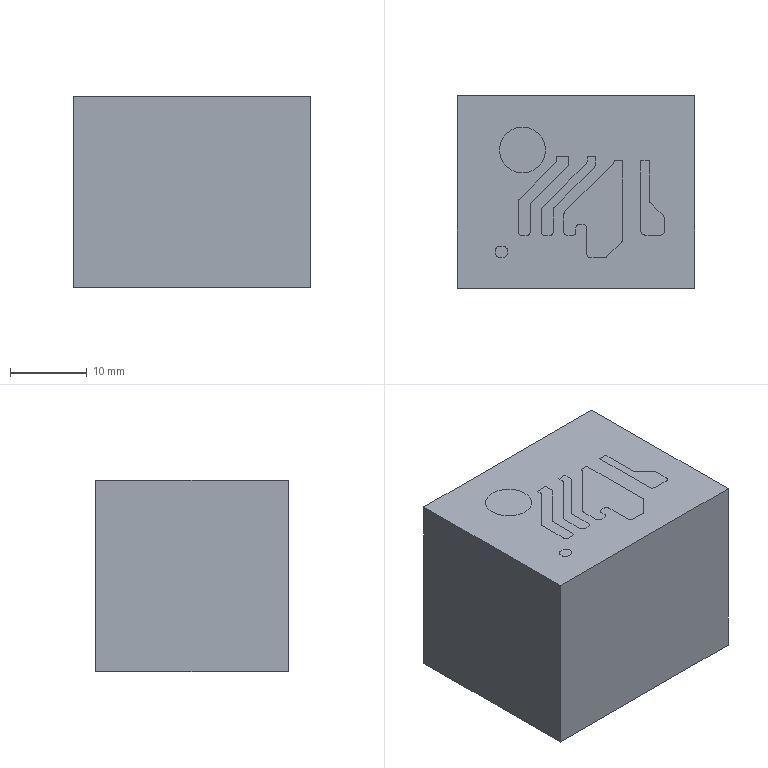Part | NX | features BREP 2 | 2 solids | 108 faces | box 31.003 x 25.176 x 25 mm | volume 28901 mm3 | plane 63 | cylinder 45 | commonest cylinder face diameters 1.1 x21 7.1 x14 0.9 x8 6 x1 8.1 x1